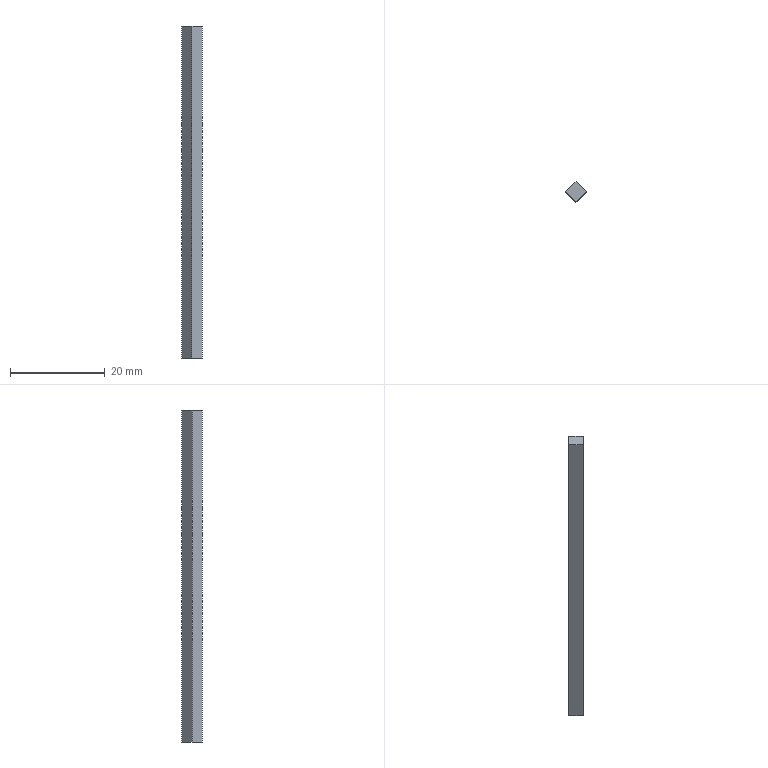Part | NX | 1 solid | 6 faces | box 4.243 x 4.243 x 70 mm | volume 630 mm3 | plane 6
STEP:
#1=CARTESIAN_POINT('',(0.,0.,0.));
#2=VERTEX_POINT('',#1);
#3=CARTESIAN_POINT('',(-2.121,-2.121,0.));
#4=VERTEX_POINT('',#3);
#5=CARTESIAN_POINT('',(0.,0.,0.));
#6=DIRECTION('',(-0.7071,-0.7071,0.));
#7=VECTOR('',#6,1000.);
#8=LINE('',#5,#7);
#9=EDGE_CURVE('',#2,#4,#8,.T.);
#10=ORIENTED_EDGE('',*,*,#9,.F.);
#11=CARTESIAN_POINT('',(2.121,-2.121,0.));
#12=VERTEX_POINT('',#11);
#13=CARTESIAN_POINT('',(2.121,-2.121,0.));
#14=DIRECTION('',(-0.7071,0.7071,0.));
#15=VECTOR('',#14,1000.);
#16=LINE('',#13,#15);
#17=EDGE_CURVE('',#12,#2,#16,.T.);
#18=ORIENTED_EDGE('',*,*,#17,.F.);
#19=CARTESIAN_POINT('',(0.,-4.243,0.));
#20=VERTEX_POINT('',#19);
#21=CARTESIAN_POINT('',(0.,-4.243,0.));
#22=DIRECTION('',(0.7071,0.7071,0.));
#23=VECTOR('',#22,1000.);
#24=LINE('',#21,#23);
#25=EDGE_CURVE('',#20,#12,#24,.T.);
#26=ORIENTED_EDGE('',*,*,#25,.F.);
#27=CARTESIAN_POINT('',(-2.121,-2.121,0.));
#28=DIRECTION('',(0.7071,-0.7071,0.));
#29=VECTOR('',#28,1000.);
#30=LINE('',#27,#29);
#31=EDGE_CURVE('',#4,#20,#30,.T.);
#32=ORIENTED_EDGE('',*,*,#31,.F.);
#33=EDGE_LOOP('',(#10,#18,#26,#32));
#34=FACE_BOUND('',#33,.T.);
#35=CARTESIAN_POINT('',(0.,0.,0.));
#36=DIRECTION('',(0.,0.,1.));
#37=DIRECTION('',(1.,0.,0.));
#38=AXIS2_PLACEMENT_3D('',#35,#36,#37);
#39=PLANE('',#38);
#40=ADVANCED_FACE('',(#34),#39,.F.);
#41=ORIENTED_EDGE('',*,*,#9,.T.);
#42=CARTESIAN_POINT('',(-2.121,-2.121,70.));
#43=VERTEX_POINT('',#42);
#44=CARTESIAN_POINT('',(-2.121,-2.121,70.));
#45=DIRECTION('',(0.,0.,-1.));
#46=VECTOR('',#45,1000.);
#47=LINE('',#44,#46);
#48=EDGE_CURVE('',#43,#4,#47,.T.);
#49=ORIENTED_EDGE('',*,*,#48,.F.);
#50=CARTESIAN_POINT('',(0.,0.,70.));
#51=VERTEX_POINT('',#50);
#52=CARTESIAN_POINT('',(-2.121,-2.121,70.));
#53=DIRECTION('',(0.7071,0.7071,0.));
#54=VECTOR('',#53,1000.);
#55=LINE('',#52,#54);
#56=EDGE_CURVE('',#43,#51,#55,.T.);
#57=ORIENTED_EDGE('',*,*,#56,.T.);
#58=CARTESIAN_POINT('',(0.,0.,70.));
#59=DIRECTION('',(0.,0.,-1.));
#60=VECTOR('',#59,1000.);
#61=LINE('',#58,#60);
#62=EDGE_CURVE('',#51,#2,#61,.T.);
#63=ORIENTED_EDGE('',*,*,#62,.T.);
#64=EDGE_LOOP('',(#41,#49,#57,#63));
#65=FACE_BOUND('',#64,.T.);
#66=CARTESIAN_POINT('',(0.,0.,0.));
#67=DIRECTION('',(-0.7071,0.7071,0.));
#68=DIRECTION('',(0.,0.,1.));
#69=AXIS2_PLACEMENT_3D('',#66,#67,#68);
#70=PLANE('',#69);
#71=ADVANCED_FACE('',(#65),#70,.T.);
#72=ORIENTED_EDGE('',*,*,#17,.T.);
#73=ORIENTED_EDGE('',*,*,#62,.F.);
#74=CARTESIAN_POINT('',(2.121,-2.121,70.));
#75=VERTEX_POINT('',#74);
#76=CARTESIAN_POINT('',(0.,0.,70.));
#77=DIRECTION('',(0.7071,-0.7071,0.));
#78=VECTOR('',#77,1000.);
#79=LINE('',#76,#78);
#80=EDGE_CURVE('',#51,#75,#79,.T.);
#81=ORIENTED_EDGE('',*,*,#80,.T.);
#82=CARTESIAN_POINT('',(2.121,-2.121,70.));
#83=DIRECTION('',(0.,0.,-1.));
#84=VECTOR('',#83,1000.);
#85=LINE('',#82,#84);
#86=EDGE_CURVE('',#75,#12,#85,.T.);
#87=ORIENTED_EDGE('',*,*,#86,.T.);
#88=EDGE_LOOP('',(#72,#73,#81,#87));
#89=FACE_BOUND('',#88,.T.);
#90=CARTESIAN_POINT('',(2.121,-2.121,0.));
#91=DIRECTION('',(0.7071,0.7071,0.));
#92=DIRECTION('',(0.,0.,-1.));
#93=AXIS2_PLACEMENT_3D('',#90,#91,#92);
#94=PLANE('',#93);
#95=ADVANCED_FACE('',(#89),#94,.T.);
#96=ORIENTED_EDGE('',*,*,#25,.T.);
#97=ORIENTED_EDGE('',*,*,#86,.F.);
#98=CARTESIAN_POINT('',(0.,-4.243,70.));
#99=VERTEX_POINT('',#98);
#100=CARTESIAN_POINT('',(2.121,-2.121,70.));
#101=DIRECTION('',(-0.7071,-0.7071,0.));
#102=VECTOR('',#101,1000.);
#103=LINE('',#100,#102);
#104=EDGE_CURVE('',#75,#99,#103,.T.);
#105=ORIENTED_EDGE('',*,*,#104,.T.);
#106=CARTESIAN_POINT('',(0.,-4.243,70.));
#107=DIRECTION('',(0.,0.,-1.));
#108=VECTOR('',#107,1000.);
#109=LINE('',#106,#108);
#110=EDGE_CURVE('',#99,#20,#109,.T.);
#111=ORIENTED_EDGE('',*,*,#110,.T.);
#112=EDGE_LOOP('',(#96,#97,#105,#111));
#113=FACE_BOUND('',#112,.T.);
#114=CARTESIAN_POINT('',(0.,-4.243,0.));
#115=DIRECTION('',(0.7071,-0.7071,0.));
#116=DIRECTION('',(0.,0.,-1.));
#117=AXIS2_PLACEMENT_3D('',#114,#115,#116);
#118=PLANE('',#117);
#119=ADVANCED_FACE('',(#113),#118,.T.);
#120=ORIENTED_EDGE('',*,*,#31,.T.);
#121=ORIENTED_EDGE('',*,*,#110,.F.);
#122=CARTESIAN_POINT('',(0.,-4.243,70.));
#123=DIRECTION('',(-0.7071,0.7071,0.));
#124=VECTOR('',#123,1000.);
#125=LINE('',#122,#124);
#126=EDGE_CURVE('',#99,#43,#125,.T.);
#127=ORIENTED_EDGE('',*,*,#126,.T.);
#128=ORIENTED_EDGE('',*,*,#48,.T.);
#129=EDGE_LOOP('',(#120,#121,#127,#128));
#130=FACE_BOUND('',#129,.T.);
#131=CARTESIAN_POINT('',(-2.121,-2.121,0.));
#132=DIRECTION('',(-0.7071,-0.7071,0.));
#133=DIRECTION('',(-0.7071,0.7071,0.));
#134=AXIS2_PLACEMENT_3D('',#131,#132,#133);
#135=PLANE('',#134);
#136=ADVANCED_FACE('',(#130),#135,.T.);
#137=ORIENTED_EDGE('',*,*,#56,.F.);
#138=ORIENTED_EDGE('',*,*,#126,.F.);
#139=ORIENTED_EDGE('',*,*,#104,.F.);
#140=ORIENTED_EDGE('',*,*,#80,.F.);
#141=EDGE_LOOP('',(#137,#138,#139,#140));
#142=FACE_BOUND('',#141,.T.);
#143=CARTESIAN_POINT('',(0.,0.,70.));
#144=DIRECTION('',(0.,0.,1.));
#145=DIRECTION('',(1.,0.,0.));
#146=AXIS2_PLACEMENT_3D('',#143,#144,#145);
#147=PLANE('',#146);
#148=ADVANCED_FACE('',(#142),#147,.T.);
#149=CLOSED_SHELL('',(#40,#71,#95,#119,#136,#148));
#150=MANIFOLD_SOLID_BREP('',#149);
#151=(LENGTH_UNIT()NAMED_UNIT(*)SI_UNIT(.MILLI.,.METRE.));
#152=UNCERTAINTY_MEASURE_WITH_UNIT(LENGTH_MEASURE(0.00001),#151,'','');
#153=(NAMED_UNIT(*)PLANE_ANGLE_UNIT()SI_UNIT($,.RADIAN.));
#154=(NAMED_UNIT(*)SI_UNIT($,.STERADIAN.)SOLID_ANGLE_UNIT());
#155=(GEOMETRIC_REPRESENTATION_CONTEXT(3)GLOBAL_UNCERTAINTY_ASSIGNED_CONTEXT((#152))GLOBAL_UNIT_ASSIGNED_CONTEXT((#151,#153,#154))REPRESENTATION_CONTEXT('',''));
#156=ADVANCED_BREP_SHAPE_REPRESENTATION('',(#150),#155);